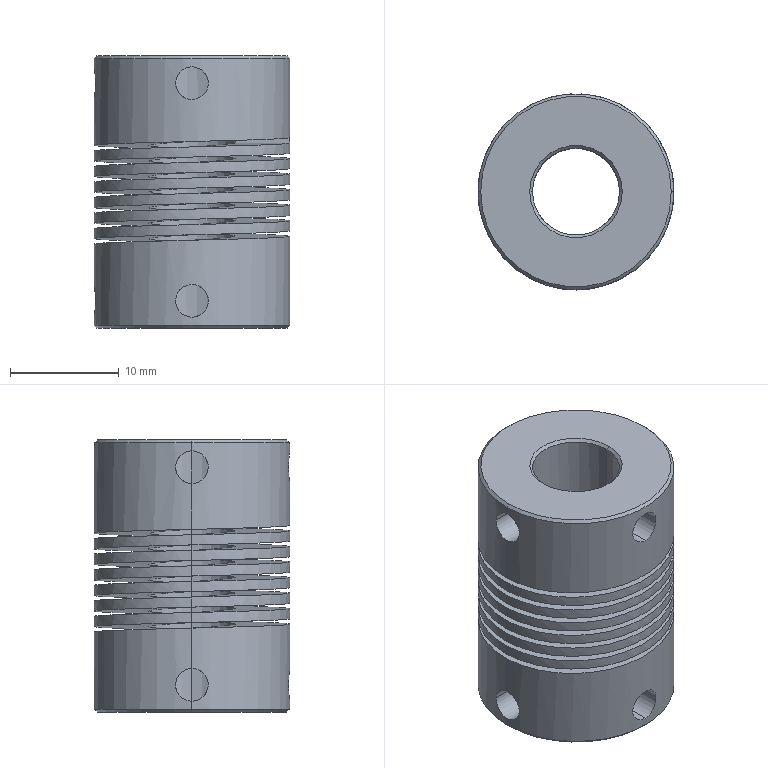Part | SolidWorks | features ICE 2, Chamfer 1, CirPattern 1, Extrusion 1, SweepCut 1 | 1 solid | 54 faces | box 18 x 18 x 25 mm | volume 4243 mm3 | cylinder 40 | cone 8 | plane 4 | spline 2 | commonest cylinder face diameters 8 x16 18 x16 3 x8